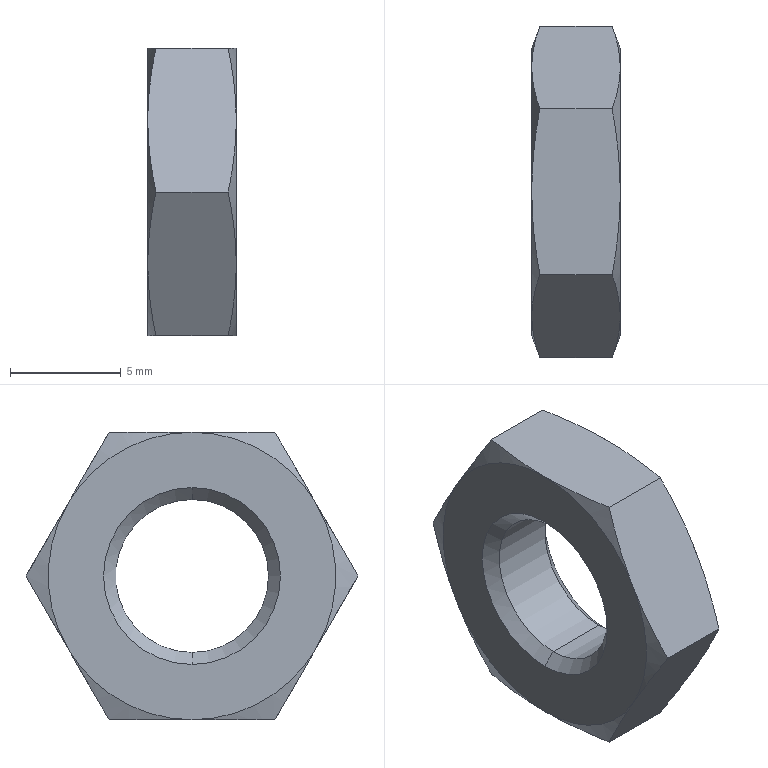Part | 1 solid | 26 faces | box 4 x 15.011 x 13 mm | volume 425.413 mm3 | cone 16 | plane 8 | cylinder 2 | commonest cylinder face diameters 6.917 x2
STEP:
#1=CARTESIAN_POINT('',(0.,0.,0.));
#2=DIRECTION('',(0.,0.,1.));
#3=DIRECTION('',(1.,0.,0.));
#4=AXIS2_PLACEMENT_3D('',#1,#2,#3);
#5=CARTESIAN_POINT('',(-291.373,167.371,-206.624));
#6=VERTEX_POINT('',#5);
#7=CARTESIAN_POINT('',(-291.007,165.494,-203.374));
#8=VERTEX_POINT('',#7);
#9=CARTESIAN_POINT('',(-291.373,167.371,-206.624));
#10=CARTESIAN_POINT('',(-291.373,166.5,-205.116));
#11=CARTESIAN_POINT('',(-291.007,165.494,-203.374));
#12=(BOUNDED_CURVE()B_SPLINE_CURVE(2,(#9,#10,#11),.UNSPECIFIED.,.F.,.U.)B_SPLINE_CURVE_WITH_KNOTS((3,3),(0.,3.786),.UNSPECIFIED.)CURVE()GEOMETRIC_REPRESENTATION_ITEM()RATIONAL_B_SPLINE_CURVE((1.,1.043,1.01))REPRESENTATION_ITEM(''));
#13=EDGE_CURVE('',#6,#8,#12,.T.);
#14=ORIENTED_EDGE('',*,*,#13,.T.);
#15=CARTESIAN_POINT('',(-291.373,167.371,-200.124));
#16=VERTEX_POINT('',#15);
#17=CARTESIAN_POINT('',(-291.007,165.494,-203.374));
#18=CARTESIAN_POINT('',(-291.373,166.5,-201.633));
#19=CARTESIAN_POINT('',(-291.373,167.371,-200.124));
#20=(BOUNDED_CURVE()B_SPLINE_CURVE(2,(#17,#18,#19),.UNSPECIFIED.,.F.,.U.)B_SPLINE_CURVE_WITH_KNOTS((3,3),(0.,3.786),.UNSPECIFIED.)CURVE()GEOMETRIC_REPRESENTATION_ITEM()RATIONAL_B_SPLINE_CURVE((1.01,1.043,1.))REPRESENTATION_ITEM(''));
#21=EDGE_CURVE('',#8,#16,#20,.T.);
#22=ORIENTED_EDGE('',*,*,#21,.T.);
#23=CARTESIAN_POINT('',(-291.373,173.,-203.374));
#24=DIRECTION('',(1.,0.,0.));
#25=DIRECTION('',(0.,-1.,0.));
#26=AXIS2_PLACEMENT_3D('',#23,#24,#25);
#27=CIRCLE('',#26,6.5);
#28=EDGE_CURVE('',#16,#6,#27,.T.);
#29=ORIENTED_EDGE('',*,*,#28,.T.);
#30=EDGE_LOOP('',(#14,#22,#29));
#31=FACE_OUTER_BOUND('',#30,.T.);
#32=CARTESIAN_POINT('',(-291.137,173.,-203.374));
#33=DIRECTION('',(1.,0.,0.));
#34=DIRECTION('',(0.,1.,0.));
#35=AXIS2_PLACEMENT_3D('',#32,#33,#34);
#36=CONICAL_SURFACE('',#35,7.15,1.222);
#37=ADVANCED_FACE('',(#31),#36,.T.);
#38=CARTESIAN_POINT('',(-287.373,167.371,-206.624));
#39=VERTEX_POINT('',#38);
#40=CARTESIAN_POINT('',(-287.739,169.247,-209.874));
#41=VERTEX_POINT('',#40);
#42=CARTESIAN_POINT('',(-287.373,167.371,-206.624));
#43=CARTESIAN_POINT('',(-287.373,168.242,-208.133));
#44=CARTESIAN_POINT('',(-287.739,169.247,-209.874));
#45=(BOUNDED_CURVE()B_SPLINE_CURVE(2,(#42,#43,#44),.UNSPECIFIED.,.F.,.U.)B_SPLINE_CURVE_WITH_KNOTS((3,3),(0.,3.786),.UNSPECIFIED.)CURVE()GEOMETRIC_REPRESENTATION_ITEM()RATIONAL_B_SPLINE_CURVE((1.,1.043,1.01))REPRESENTATION_ITEM(''));
#46=EDGE_CURVE('',#39,#41,#45,.T.);
#47=ORIENTED_EDGE('',*,*,#46,.F.);
#48=CARTESIAN_POINT('',(-287.739,165.494,-203.374));
#49=VERTEX_POINT('',#48);
#50=CARTESIAN_POINT('',(-287.739,165.494,-203.374));
#51=CARTESIAN_POINT('',(-287.373,166.5,-205.116));
#52=CARTESIAN_POINT('',(-287.373,167.371,-206.624));
#53=(BOUNDED_CURVE()B_SPLINE_CURVE(2,(#50,#51,#52),.UNSPECIFIED.,.F.,.U.)B_SPLINE_CURVE_WITH_KNOTS((3,3),(0.,3.786),.UNSPECIFIED.)CURVE()GEOMETRIC_REPRESENTATION_ITEM()RATIONAL_B_SPLINE_CURVE((1.01,1.043,1.))REPRESENTATION_ITEM(''));
#54=EDGE_CURVE('',#49,#39,#53,.T.);
#55=ORIENTED_EDGE('',*,*,#54,.F.);
#56=CARTESIAN_POINT('',(-293.373,165.494,-203.374));
#57=DIRECTION('',(1.,0.,0.));
#58=VECTOR('',#57,1.);
#59=LINE('',#56,#58);
#60=EDGE_CURVE('',#8,#49,#59,.T.);
#61=ORIENTED_EDGE('',*,*,#60,.F.);
#62=ORIENTED_EDGE('',*,*,#13,.F.);
#63=CARTESIAN_POINT('',(-291.007,169.247,-209.874));
#64=VERTEX_POINT('',#63);
#65=CARTESIAN_POINT('',(-291.007,169.247,-209.874));
#66=CARTESIAN_POINT('',(-291.373,168.242,-208.133));
#67=CARTESIAN_POINT('',(-291.373,167.371,-206.624));
#68=(BOUNDED_CURVE()B_SPLINE_CURVE(2,(#65,#66,#67),.UNSPECIFIED.,.F.,.U.)B_SPLINE_CURVE_WITH_KNOTS((3,3),(0.,3.786),.UNSPECIFIED.)CURVE()GEOMETRIC_REPRESENTATION_ITEM()RATIONAL_B_SPLINE_CURVE((1.01,1.043,1.))REPRESENTATION_ITEM(''));
#69=EDGE_CURVE('',#64,#6,#68,.T.);
#70=ORIENTED_EDGE('',*,*,#69,.F.);
#71=CARTESIAN_POINT('',(-293.373,169.247,-209.874));
#72=DIRECTION('',(1.,0.,0.));
#73=VECTOR('',#72,1.);
#74=LINE('',#71,#73);
#75=EDGE_CURVE('',#64,#41,#74,.T.);
#76=ORIENTED_EDGE('',*,*,#75,.T.);
#77=EDGE_LOOP('',(#47,#55,#61,#62,#70,#76));
#78=FACE_OUTER_BOUND('',#77,.T.);
#79=CARTESIAN_POINT('',(-293.373,165.494,-203.374));
#80=DIRECTION('',(0.,0.866,0.5));
#81=DIRECTION('',(0.,-0.5,0.866));
#82=AXIS2_PLACEMENT_3D('',#79,#80,#81);
#83=PLANE('',#82);
#84=ADVANCED_FACE('',(#78),#83,.F.);
#85=CARTESIAN_POINT('',(-287.373,173.,-209.874));
#86=VERTEX_POINT('',#85);
#87=CARTESIAN_POINT('',(-287.739,176.753,-209.874));
#88=VERTEX_POINT('',#87);
#89=CARTESIAN_POINT('',(-287.373,173.,-209.874));
#90=CARTESIAN_POINT('',(-287.373,174.742,-209.874));
#91=CARTESIAN_POINT('',(-287.739,176.753,-209.874));
#92=(BOUNDED_CURVE()B_SPLINE_CURVE(2,(#89,#90,#91),.UNSPECIFIED.,.F.,.U.)B_SPLINE_CURVE_WITH_KNOTS((3,3),(0.,3.786),.UNSPECIFIED.)CURVE()GEOMETRIC_REPRESENTATION_ITEM()RATIONAL_B_SPLINE_CURVE((1.,1.043,1.01))REPRESENTATION_ITEM(''));
#93=EDGE_CURVE('',#86,#88,#92,.T.);
#94=ORIENTED_EDGE('',*,*,#93,.F.);
#95=CARTESIAN_POINT('',(-287.739,169.247,-209.874));
#96=CARTESIAN_POINT('',(-287.373,171.258,-209.874));
#97=CARTESIAN_POINT('',(-287.373,173.,-209.874));
#98=(BOUNDED_CURVE()B_SPLINE_CURVE(2,(#95,#96,#97),.UNSPECIFIED.,.F.,.U.)B_SPLINE_CURVE_WITH_KNOTS((3,3),(0.,3.786),.UNSPECIFIED.)CURVE()GEOMETRIC_REPRESENTATION_ITEM()RATIONAL_B_SPLINE_CURVE((1.01,1.043,1.))REPRESENTATION_ITEM(''));
#99=EDGE_CURVE('',#41,#86,#98,.T.);
#100=ORIENTED_EDGE('',*,*,#99,.F.);
#101=ORIENTED_EDGE('',*,*,#75,.F.);
#102=CARTESIAN_POINT('',(-291.373,173.,-209.874));
#103=VERTEX_POINT('',#102);
#104=CARTESIAN_POINT('',(-291.373,173.,-209.874));
#105=CARTESIAN_POINT('',(-291.373,171.258,-209.874));
#106=CARTESIAN_POINT('',(-291.007,169.247,-209.874));
#107=(BOUNDED_CURVE()B_SPLINE_CURVE(2,(#104,#105,#106),.UNSPECIFIED.,.F.,.U.)B_SPLINE_CURVE_WITH_KNOTS((3,3),(0.,3.786),.UNSPECIFIED.)CURVE()GEOMETRIC_REPRESENTATION_ITEM()RATIONAL_B_SPLINE_CURVE((1.,1.043,1.01))REPRESENTATION_ITEM(''));
#108=EDGE_CURVE('',#103,#64,#107,.T.);
#109=ORIENTED_EDGE('',*,*,#108,.F.);
#110=CARTESIAN_POINT('',(-291.007,176.753,-209.874));
#111=VERTEX_POINT('',#110);
#112=CARTESIAN_POINT('',(-291.007,176.753,-209.874));
#113=CARTESIAN_POINT('',(-291.373,174.742,-209.874));
#114=CARTESIAN_POINT('',(-291.373,173.,-209.874));
#115=(BOUNDED_CURVE()B_SPLINE_CURVE(2,(#112,#113,#114),.UNSPECIFIED.,.F.,.U.)B_SPLINE_CURVE_WITH_KNOTS((3,3),(0.,3.786),.UNSPECIFIED.)CURVE()GEOMETRIC_REPRESENTATION_ITEM()RATIONAL_B_SPLINE_CURVE((1.01,1.043,1.))REPRESENTATION_ITEM(''));
#116=EDGE_CURVE('',#111,#103,#115,.T.);
#117=ORIENTED_EDGE('',*,*,#116,.F.);
#118=CARTESIAN_POINT('',(-293.373,176.753,-209.874));
#119=DIRECTION('',(1.,0.,0.));
#120=VECTOR('',#119,1.);
#121=LINE('',#118,#120);
#122=EDGE_CURVE('',#111,#88,#121,.T.);
#123=ORIENTED_EDGE('',*,*,#122,.T.);
#124=EDGE_LOOP('',(#94,#100,#101,#109,#117,#123));
#125=FACE_OUTER_BOUND('',#124,.T.);
#126=CARTESIAN_POINT('',(-293.373,169.247,-209.874));
#127=DIRECTION('',(0.,0.,1.));
#128=DIRECTION('',(0.,-1.,0.));
#129=AXIS2_PLACEMENT_3D('',#126,#127,#128);
#130=PLANE('',#129);
#131=ADVANCED_FACE('',(#125),#130,.F.);
#132=CARTESIAN_POINT('',(-287.373,178.629,-206.624));
#133=VERTEX_POINT('',#132);
#134=CARTESIAN_POINT('',(-287.739,180.506,-203.374));
#135=VERTEX_POINT('',#134);
#136=CARTESIAN_POINT('',(-287.373,178.629,-206.624));
#137=CARTESIAN_POINT('',(-287.373,179.5,-205.116));
#138=CARTESIAN_POINT('',(-287.739,180.506,-203.374));
#139=(BOUNDED_CURVE()B_SPLINE_CURVE(2,(#136,#137,#138),.UNSPECIFIED.,.F.,.U.)B_SPLINE_CURVE_WITH_KNOTS((3,3),(0.,3.786),.UNSPECIFIED.)CURVE()GEOMETRIC_REPRESENTATION_ITEM()RATIONAL_B_SPLINE_CURVE((1.,1.043,1.01))REPRESENTATION_ITEM(''));
#140=EDGE_CURVE('',#133,#135,#139,.T.);
#141=ORIENTED_EDGE('',*,*,#140,.F.);
#142=CARTESIAN_POINT('',(-287.739,176.753,-209.874));
#143=CARTESIAN_POINT('',(-287.373,177.758,-208.133));
#144=CARTESIAN_POINT('',(-287.373,178.629,-206.624));
#145=(BOUNDED_CURVE()B_SPLINE_CURVE(2,(#142,#143,#144),.UNSPECIFIED.,.F.,.U.)B_SPLINE_CURVE_WITH_KNOTS((3,3),(0.,3.786),.UNSPECIFIED.)CURVE()GEOMETRIC_REPRESENTATION_ITEM()RATIONAL_B_SPLINE_CURVE((1.01,1.043,1.))REPRESENTATION_ITEM(''));
#146=EDGE_CURVE('',#88,#133,#145,.T.);
#147=ORIENTED_EDGE('',*,*,#146,.F.);
#148=ORIENTED_EDGE('',*,*,#122,.F.);
#149=CARTESIAN_POINT('',(-291.373,178.629,-206.624));
#150=VERTEX_POINT('',#149);
#151=CARTESIAN_POINT('',(-291.373,178.629,-206.624));
#152=CARTESIAN_POINT('',(-291.373,177.758,-208.133));
#153=CARTESIAN_POINT('',(-291.007,176.753,-209.874));
#154=(BOUNDED_CURVE()B_SPLINE_CURVE(2,(#151,#152,#153),.UNSPECIFIED.,.F.,.U.)B_SPLINE_CURVE_WITH_KNOTS((3,3),(0.,3.786),.UNSPECIFIED.)CURVE()GEOMETRIC_REPRESENTATION_ITEM()RATIONAL_B_SPLINE_CURVE((1.,1.043,1.01))REPRESENTATION_ITEM(''));
#155=EDGE_CURVE('',#150,#111,#154,.T.);
#156=ORIENTED_EDGE('',*,*,#155,.F.);
#157=CARTESIAN_POINT('',(-291.007,180.506,-203.374));
#158=VERTEX_POINT('',#157);
#159=CARTESIAN_POINT('',(-291.007,180.506,-203.374));
#160=CARTESIAN_POINT('',(-291.373,179.5,-205.116));
#161=CARTESIAN_POINT('',(-291.373,178.629,-206.624));
#162=(BOUNDED_CURVE()B_SPLINE_CURVE(2,(#159,#160,#161),.UNSPECIFIED.,.F.,.U.)B_SPLINE_CURVE_WITH_KNOTS((3,3),(0.,3.786),.UNSPECIFIED.)CURVE()GEOMETRIC_REPRESENTATION_ITEM()RATIONAL_B_SPLINE_CURVE((1.01,1.043,1.))REPRESENTATION_ITEM(''));
#163=EDGE_CURVE('',#158,#150,#162,.T.);
#164=ORIENTED_EDGE('',*,*,#163,.F.);
#165=CARTESIAN_POINT('',(-293.373,180.506,-203.374));
#166=DIRECTION('',(1.,0.,0.));
#167=VECTOR('',#166,1.);
#168=LINE('',#165,#167);
#169=EDGE_CURVE('',#158,#135,#168,.T.);
#170=ORIENTED_EDGE('',*,*,#169,.T.);
#171=EDGE_LOOP('',(#141,#147,#148,#156,#164,#170));
#172=FACE_OUTER_BOUND('',#171,.T.);
#173=CARTESIAN_POINT('',(-293.373,176.753,-209.874));
#174=DIRECTION('',(0.,-0.866,0.5));
#175=DIRECTION('',(0.,-0.5,-0.866));
#176=AXIS2_PLACEMENT_3D('',#173,#174,#175);
#177=PLANE('',#176);
#178=ADVANCED_FACE('',(#172),#177,.F.);
#179=CARTESIAN_POINT('',(-287.373,178.629,-200.124));
#180=VERTEX_POINT('',#179);
#181=CARTESIAN_POINT('',(-287.739,180.506,-203.374));
#182=CARTESIAN_POINT('',(-287.373,179.5,-201.633));
#183=CARTESIAN_POINT('',(-287.373,178.629,-200.124));
#184=(BOUNDED_CURVE()B_SPLINE_CURVE(2,(#181,#182,#183),.UNSPECIFIED.,.F.,.U.)B_SPLINE_CURVE_WITH_KNOTS((3,3),(0.,3.786),.UNSPECIFIED.)CURVE()GEOMETRIC_REPRESENTATION_ITEM()RATIONAL_B_SPLINE_CURVE((1.01,1.043,1.))REPRESENTATION_ITEM(''));
#185=EDGE_CURVE('',#135,#180,#184,.T.);
#186=ORIENTED_EDGE('',*,*,#185,.F.);
#187=ORIENTED_EDGE('',*,*,#169,.F.);
#188=CARTESIAN_POINT('',(-291.373,178.629,-200.124));
#189=VERTEX_POINT('',#188);
#190=CARTESIAN_POINT('',(-291.373,178.629,-200.124));
#191=CARTESIAN_POINT('',(-291.373,179.5,-201.633));
#192=CARTESIAN_POINT('',(-291.007,180.506,-203.374));
#193=(BOUNDED_CURVE()B_SPLINE_CURVE(2,(#190,#191,#192),.UNSPECIFIED.,.F.,.U.)B_SPLINE_CURVE_WITH_KNOTS((3,3),(0.,3.786),.UNSPECIFIED.)CURVE()GEOMETRIC_REPRESENTATION_ITEM()RATIONAL_B_SPLINE_CURVE((1.,1.043,1.01))REPRESENTATION_ITEM(''));
#194=EDGE_CURVE('',#189,#158,#193,.T.);
#195=ORIENTED_EDGE('',*,*,#194,.F.);
#196=CARTESIAN_POINT('',(-291.007,176.753,-196.874));
#197=VERTEX_POINT('',#196);
#198=CARTESIAN_POINT('',(-291.007,176.753,-196.874));
#199=CARTESIAN_POINT('',(-291.373,177.758,-198.616));
#200=CARTESIAN_POINT('',(-291.373,178.629,-200.124));
#201=(BOUNDED_CURVE()B_SPLINE_CURVE(2,(#198,#199,#200),.UNSPECIFIED.,.F.,.U.)B_SPLINE_CURVE_WITH_KNOTS((3,3),(0.,3.786),.UNSPECIFIED.)CURVE()GEOMETRIC_REPRESENTATION_ITEM()RATIONAL_B_SPLINE_CURVE((1.01,1.043,1.))REPRESENTATION_ITEM(''));
#202=EDGE_CURVE('',#197,#189,#201,.T.);
#203=ORIENTED_EDGE('',*,*,#202,.F.);
#204=CARTESIAN_POINT('',(-287.739,176.753,-196.874));
#205=VERTEX_POINT('',#204);
#206=CARTESIAN_POINT('',(-293.373,176.753,-196.874));
#207=DIRECTION('',(1.,0.,0.));
#208=VECTOR('',#207,1.);
#209=LINE('',#206,#208);
#210=EDGE_CURVE('',#197,#205,#209,.T.);
#211=ORIENTED_EDGE('',*,*,#210,.T.);
#212=CARTESIAN_POINT('',(-287.373,178.629,-200.124));
#213=CARTESIAN_POINT('',(-287.373,177.758,-198.616));
#214=CARTESIAN_POINT('',(-287.739,176.753,-196.874));
#215=(BOUNDED_CURVE()B_SPLINE_CURVE(2,(#212,#213,#214),.UNSPECIFIED.,.F.,.U.)B_SPLINE_CURVE_WITH_KNOTS((3,3),(0.,3.786),.UNSPECIFIED.)CURVE()GEOMETRIC_REPRESENTATION_ITEM()RATIONAL_B_SPLINE_CURVE((1.,1.043,1.01))REPRESENTATION_ITEM(''));
#216=EDGE_CURVE('',#180,#205,#215,.T.);
#217=ORIENTED_EDGE('',*,*,#216,.F.);
#218=EDGE_LOOP('',(#186,#187,#195,#203,#211,#217));
#219=FACE_OUTER_BOUND('',#218,.T.);
#220=CARTESIAN_POINT('',(-293.373,180.506,-203.374));
#221=DIRECTION('',(0.,-0.866,-0.5));
#222=DIRECTION('',(0.,0.5,-0.866));
#223=AXIS2_PLACEMENT_3D('',#220,#221,#222);
#224=PLANE('',#223);
#225=ADVANCED_FACE('',(#219),#224,.F.);
#226=ORIENTED_EDGE('',*,*,#216,.T.);
#227=CARTESIAN_POINT('',(-287.373,173.,-196.874));
#228=VERTEX_POINT('',#227);
#229=CARTESIAN_POINT('',(-287.739,176.753,-196.874));
#230=CARTESIAN_POINT('',(-287.373,174.742,-196.874));
#231=CARTESIAN_POINT('',(-287.373,173.,-196.874));
#232=(BOUNDED_CURVE()B_SPLINE_CURVE(2,(#229,#230,#231),.UNSPECIFIED.,.F.,.U.)B_SPLINE_CURVE_WITH_KNOTS((3,3),(0.,3.786),.UNSPECIFIED.)CURVE()GEOMETRIC_REPRESENTATION_ITEM()RATIONAL_B_SPLINE_CURVE((1.01,1.043,1.))REPRESENTATION_ITEM(''));
#233=EDGE_CURVE('',#205,#228,#232,.T.);
#234=ORIENTED_EDGE('',*,*,#233,.T.);
#235=CARTESIAN_POINT('',(-287.373,173.,-203.374));
#236=DIRECTION('',(1.,0.,0.));
#237=DIRECTION('',(0.,-1.,0.));
#238=AXIS2_PLACEMENT_3D('',#235,#236,#237);
#239=CIRCLE('',#238,6.5);
#240=EDGE_CURVE('',#180,#228,#239,.T.);
#241=ORIENTED_EDGE('',*,*,#240,.F.);
#242=EDGE_LOOP('',(#226,#234,#241));
#243=FACE_OUTER_BOUND('',#242,.T.);
#244=CARTESIAN_POINT('',(-287.61,173.,-203.374));
#245=DIRECTION('',(-1.,0.,0.));
#246=DIRECTION('',(0.,-0.5,-0.866));
#247=AXIS2_PLACEMENT_3D('',#244,#245,#246);
#248=CONICAL_SURFACE('',#247,7.15,1.222);
#249=ADVANCED_FACE('',(#243),#248,.T.);
#250=CARTESIAN_POINT('',(-287.373,169.,-203.374));
#251=VERTEX_POINT('',#250);
#252=CARTESIAN_POINT('',(-287.373,173.,-199.374));
#253=VERTEX_POINT('',#252);
#254=CARTESIAN_POINT('',(-287.373,173.,-203.374));
#255=DIRECTION('',(-1.,0.,0.));
#256=DIRECTION('',(0.,-1.,0.));
#257=AXIS2_PLACEMENT_3D('',#254,#255,#256);
#258=CIRCLE('',#257,4.);
#259=EDGE_CURVE('',#251,#253,#258,.T.);
#260=ORIENTED_EDGE('',*,*,#259,.T.);
#261=CARTESIAN_POINT('',(-287.373,173.,-207.374));
#262=VERTEX_POINT('',#261);
#263=CARTESIAN_POINT('',(-287.373,173.,-203.374));
#264=DIRECTION('',(-1.,0.,0.));
#265=DIRECTION('',(0.,-1.,0.));
#266=AXIS2_PLACEMENT_3D('',#263,#264,#265);
#267=CIRCLE('',#266,4.);
#268=EDGE_CURVE('',#253,#262,#267,.T.);
#269=ORIENTED_EDGE('',*,*,#268,.T.);
#270=CARTESIAN_POINT('',(-287.373,173.,-203.374));
#271=DIRECTION('',(-1.,0.,0.));
#272=DIRECTION('',(0.,-1.,0.));
#273=AXIS2_PLACEMENT_3D('',#270,#271,#272);
#274=CIRCLE('',#273,4.);
#275=EDGE_CURVE('',#262,#251,#274,.T.);
#276=ORIENTED_EDGE('',*,*,#275,.T.);
#277=EDGE_LOOP('',(#260,#269,#276));
#278=FACE_BOUND('',#277,.T.);
#279=CARTESIAN_POINT('',(-287.373,167.371,-200.124));
#280=VERTEX_POINT('',#279);
#281=CARTESIAN_POINT('',(-287.373,173.,-203.374));
#282=DIRECTION('',(1.,0.,0.));
#283=DIRECTION('',(0.,-1.,0.));
#284=AXIS2_PLACEMENT_3D('',#281,#282,#283);
#285=CIRCLE('',#284,6.5);
#286=EDGE_CURVE('',#228,#280,#285,.T.);
#287=ORIENTED_EDGE('',*,*,#286,.T.);
#288=CARTESIAN_POINT('',(-287.373,173.,-203.374));
#289=DIRECTION('',(1.,0.,0.));
#290=DIRECTION('',(0.,-1.,0.));
#291=AXIS2_PLACEMENT_3D('',#288,#289,#290);
#292=CIRCLE('',#291,6.5);
#293=EDGE_CURVE('',#280,#39,#292,.T.);
#294=ORIENTED_EDGE('',*,*,#293,.T.);
#295=CARTESIAN_POINT('',(-287.373,173.,-203.374));
#296=DIRECTION('',(1.,0.,0.));
#297=DIRECTION('',(0.,-1.,0.));
#298=AXIS2_PLACEMENT_3D('',#295,#296,#297);
#299=CIRCLE('',#298,6.5);
#300=EDGE_CURVE('',#39,#86,#299,.T.);
#301=ORIENTED_EDGE('',*,*,#300,.T.);
#302=CARTESIAN_POINT('',(-287.373,173.,-203.374));
#303=DIRECTION('',(1.,0.,0.));
#304=DIRECTION('',(0.,-1.,0.));
#305=AXIS2_PLACEMENT_3D('',#302,#303,#304);
#306=CIRCLE('',#305,6.5);
#307=EDGE_CURVE('',#86,#133,#306,.T.);
#308=ORIENTED_EDGE('',*,*,#307,.T.);
#309=CARTESIAN_POINT('',(-287.373,173.,-203.374));
#310=DIRECTION('',(1.,0.,0.));
#311=DIRECTION('',(0.,-1.,0.));
#312=AXIS2_PLACEMENT_3D('',#309,#310,#311);
#313=CIRCLE('',#312,6.5);
#314=EDGE_CURVE('',#133,#180,#313,.T.);
#315=ORIENTED_EDGE('',*,*,#314,.T.);
#316=ORIENTED_EDGE('',*,*,#240,.T.);
#317=EDGE_LOOP('',(#287,#294,#301,#308,#315,#316));
#318=FACE_OUTER_BOUND('',#317,.T.);
#319=CARTESIAN_POINT('',(-287.373,169.75,-203.374));
#320=DIRECTION('',(1.,0.,0.));
#321=DIRECTION('',(0.,-1.,0.));
#322=AXIS2_PLACEMENT_3D('',#319,#320,#321);
#323=PLANE('',#322);
#324=ADVANCED_FACE('',(#278,#318),#323,.T.);
#325=CARTESIAN_POINT('',(-287.739,169.247,-196.874));
#326=VERTEX_POINT('',#325);
#327=CARTESIAN_POINT('',(-287.373,173.,-196.874));
#328=CARTESIAN_POINT('',(-287.373,171.258,-196.874));
#329=CARTESIAN_POINT('',(-287.739,169.247,-196.874));
#330=(BOUNDED_CURVE()B_SPLINE_CURVE(2,(#327,#328,#329),.UNSPECIFIED.,.F.,.U.)B_SPLINE_CURVE_WITH_KNOTS((3,3),(0.,3.786),.UNSPECIFIED.)CURVE()GEOMETRIC_REPRESENTATION_ITEM()RATIONAL_B_SPLINE_CURVE((1.,1.043,1.01))REPRESENTATION_ITEM(''));
#331=EDGE_CURVE('',#228,#326,#330,.T.);
#332=ORIENTED_EDGE('',*,*,#331,.T.);
#333=CARTESIAN_POINT('',(-287.739,169.247,-196.874));
#334=CARTESIAN_POINT('',(-287.373,168.242,-198.616));
#335=CARTESIAN_POINT('',(-287.373,167.371,-200.124));
#336=(BOUNDED_CURVE()B_SPLINE_CURVE(2,(#333,#334,#335),.UNSPECIFIED.,.F.,.U.)B_SPLINE_CURVE_WITH_KNOTS((3,3),(0.,3.786),.UNSPECIFIED.)CURVE()GEOMETRIC_REPRESENTATION_ITEM()RATIONAL_B_SPLINE_CURVE((1.01,1.043,1.))REPRESENTATION_ITEM(''));
#337=EDGE_CURVE('',#326,#280,#336,.T.);
#338=ORIENTED_EDGE('',*,*,#337,.T.);
#339=ORIENTED_EDGE('',*,*,#286,.F.);
#340=EDGE_LOOP('',(#332,#338,#339));
#341=FACE_OUTER_BOUND('',#340,.T.);
#342=CARTESIAN_POINT('',(-287.61,173.,-203.374));
#343=DIRECTION('',(-1.,0.,0.));
#344=DIRECTION('',(0.,0.5,-0.866));
#345=AXIS2_PLACEMENT_3D('',#342,#343,#344);
#346=CONICAL_SURFACE('',#345,7.15,1.222);
#347=ADVANCED_FACE('',(#341),#346,.T.);
#348=ORIENTED_EDGE('',*,*,#337,.F.);
#349=CARTESIAN_POINT('',(-291.007,169.247,-196.874));
#350=VERTEX_POINT('',#349);
#351=CARTESIAN_POINT('',(-293.373,169.247,-196.874));
#352=DIRECTION('',(1.,0.,0.));
#353=VECTOR('',#352,1.);
#354=LINE('',#351,#353);
#355=EDGE_CURVE('',#350,#326,#354,.T.);
#356=ORIENTED_EDGE('',*,*,#355,.F.);
#357=CARTESIAN_POINT('',(-291.373,167.371,-200.124));
#358=CARTESIAN_POINT('',(-291.373,168.242,-198.616));
#359=CARTESIAN_POINT('',(-291.007,169.247,-196.874));
#360=(BOUNDED_CURVE()B_SPLINE_CURVE(2,(#357,#358,#359),.UNSPECIFIED.,.F.,.U.)B_SPLINE_CURVE_WITH_KNOTS((3,3),(0.,3.786),.UNSPECIFIED.)CURVE()GEOMETRIC_REPRESENTATION_ITEM()RATIONAL_B_SPLINE_CURVE((1.,1.043,1.01))REPRESENTATION_ITEM(''));
#361=EDGE_CURVE('',#16,#350,#360,.T.);
#362=ORIENTED_EDGE('',*,*,#361,.F.);
#363=ORIENTED_EDGE('',*,*,#21,.F.);
#364=ORIENTED_EDGE('',*,*,#60,.T.);
#365=CARTESIAN_POINT('',(-287.373,167.371,-200.124));
#366=CARTESIAN_POINT('',(-287.373,166.5,-201.633));
#367=CARTESIAN_POINT('',(-287.739,165.494,-203.374));
#368=(BOUNDED_CURVE()B_SPLINE_CURVE(2,(#365,#366,#367),.UNSPECIFIED.,.F.,.U.)B_SPLINE_CURVE_WITH_KNOTS((3,3),(0.,3.786),.UNSPECIFIED.)CURVE()GEOMETRIC_REPRESENTATION_ITEM()RATIONAL_B_SPLINE_CURVE((1.,1.043,1.01))REPRESENTATION_ITEM(''));
#369=EDGE_CURVE('',#280,#49,#368,.T.);
#370=ORIENTED_EDGE('',*,*,#369,.F.);
#371=EDGE_LOOP('',(#348,#356,#362,#363,#364,#370));
#372=FACE_OUTER_BOUND('',#371,.T.);
#373=CARTESIAN_POINT('',(-293.373,169.247,-196.874));
#374=DIRECTION('',(0.,0.866,-0.5));
#375=DIRECTION('',(0.,0.5,0.866));
#376=AXIS2_PLACEMENT_3D('',#373,#374,#375);
#377=PLANE('',#376);
#378=ADVANCED_FACE('',(#372),#377,.F.);
#379=ORIENTED_EDGE('',*,*,#293,.F.);
#380=ORIENTED_EDGE('',*,*,#369,.T.);
#381=ORIENTED_EDGE('',*,*,#54,.T.);
#382=EDGE_LOOP('',(#379,#380,#381));
#383=FACE_OUTER_BOUND('',#382,.T.);
#384=CARTESIAN_POINT('',(-287.61,173.,-203.374));
#385=DIRECTION('',(-1.,0.,0.));
#386=DIRECTION('',(0.,1.,0.));
#387=AXIS2_PLACEMENT_3D('',#384,#385,#386);
#388=CONICAL_SURFACE('',#387,7.15,1.222);
#389=ADVANCED_FACE('',(#383),#388,.T.);
#390=CARTESIAN_POINT('',(-291.373,169.,-203.374));
#391=VERTEX_POINT('',#390);
#392=CARTESIAN_POINT('',(-291.373,173.,-207.374));
#393=VERTEX_POINT('',#392);
#394=CARTESIAN_POINT('',(-291.373,173.,-203.374));
#395=DIRECTION('',(1.,0.,0.));
#396=DIRECTION('',(0.,-1.,0.));
#397=AXIS2_PLACEMENT_3D('',#394,#395,#396);
#398=CIRCLE('',#397,4.);
#399=EDGE_CURVE('',#391,#393,#398,.T.);
#400=ORIENTED_EDGE('',*,*,#399,.T.);
#401=CARTESIAN_POINT('',(-291.373,173.,-199.374));
#402=VERTEX_POINT('',#401);
#403=CARTESIAN_POINT('',(-291.373,173.,-203.374));
#404=DIRECTION('',(1.,0.,0.));
#405=DIRECTION('',(0.,-1.,0.));
#406=AXIS2_PLACEMENT_3D('',#403,#404,#405);
#407=CIRCLE('',#406,4.);
#408=EDGE_CURVE('',#393,#402,#407,.T.);
#409=ORIENTED_EDGE('',*,*,#408,.T.);
#410=CARTESIAN_POINT('',(-291.373,173.,-203.374));
#411=DIRECTION('',(1.,0.,0.));
#412=DIRECTION('',(0.,-1.,0.));
#413=AXIS2_PLACEMENT_3D('',#410,#411,#412);
#414=CIRCLE('',#413,4.);
#415=EDGE_CURVE('',#402,#391,#414,.T.);
#416=ORIENTED_EDGE('',*,*,#415,.T.);
#417=EDGE_LOOP('',(#400,#409,#416));
#418=FACE_BOUND('',#417,.T.);
#419=ORIENTED_EDGE('',*,*,#28,.F.);
#420=CARTESIAN_POINT('',(-291.373,173.,-196.874));
#421=VERTEX_POINT('',#420);
#422=CARTESIAN_POINT('',(-291.373,173.,-203.374));
#423=DIRECTION('',(1.,0.,0.));
#424=DIRECTION('',(0.,-1.,0.));
#425=AXIS2_PLACEMENT_3D('',#422,#423,#424);
#426=CIRCLE('',#425,6.5);
#427=EDGE_CURVE('',#421,#16,#426,.T.);
#428=ORIENTED_EDGE('',*,*,#427,.F.);
#429=CARTESIAN_POINT('',(-291.373,173.,-203.374));
#430=DIRECTION('',(1.,0.,0.));
#431=DIRECTION('',(0.,-1.,0.));
#432=AXIS2_PLACEMENT_3D('',#429,#430,#431);
#433=CIRCLE('',#432,6.5);
#434=EDGE_CURVE('',#189,#421,#433,.T.);
#435=ORIENTED_EDGE('',*,*,#434,.F.);
#436=CARTESIAN_POINT('',(-291.373,173.,-203.374));
#437=DIRECTION('',(1.,0.,0.));
#438=DIRECTION('',(0.,-1.,0.));
#439=AXIS2_PLACEMENT_3D('',#436,#437,#438);
#440=CIRCLE('',#439,6.5);
#441=EDGE_CURVE('',#150,#189,#440,.T.);
#442=ORIENTED_EDGE('',*,*,#441,.F.);
#443=CARTESIAN_POINT('',(-291.373,173.,-203.374));
#444=DIRECTION('',(1.,0.,0.));
#445=DIRECTION('',(0.,-1.,0.));
#446=AXIS2_PLACEMENT_3D('',#443,#444,#445);
#447=CIRCLE('',#446,6.5);
#448=EDGE_CURVE('',#103,#150,#447,.T.);
#449=ORIENTED_EDGE('',*,*,#448,.F.);
#450=CARTESIAN_POINT('',(-291.373,173.,-203.374));
#451=DIRECTION('',(1.,0.,0.));
#452=DIRECTION('',(0.,-1.,0.));
#453=AXIS2_PLACEMENT_3D('',#450,#451,#452);
#454=CIRCLE('',#453,6.5);
#455=EDGE_CURVE('',#6,#103,#454,.T.);
#456=ORIENTED_EDGE('',*,*,#455,.F.);
#457=EDGE_LOOP('',(#419,#428,#435,#442,#449,#456));
#458=FACE_OUTER_BOUND('',#457,.T.);
#459=CARTESIAN_POINT('',(-291.373,169.75,-203.374));
#460=DIRECTION('',(-1.,0.,0.));
#461=DIRECTION('',(0.,1.,0.));
#462=AXIS2_PLACEMENT_3D('',#459,#460,#461);
#463=PLANE('',#462);
#464=ADVANCED_FACE('',(#418,#458),#463,.T.);
#465=ORIENTED_EDGE('',*,*,#108,.T.);
#466=ORIENTED_EDGE('',*,*,#69,.T.);
#467=ORIENTED_EDGE('',*,*,#455,.T.);
#468=EDGE_LOOP('',(#465,#466,#467));
#469=FACE_OUTER_BOUND('',#468,.T.);
#470=CARTESIAN_POINT('',(-291.137,173.,-203.374));
#471=DIRECTION('',(1.,0.,0.));
#472=DIRECTION('',(0.,0.5,0.866));
#473=AXIS2_PLACEMENT_3D('',#470,#471,#472);
#474=CONICAL_SURFACE('',#473,7.15,1.222);
#475=ADVANCED_FACE('',(#469),#474,.T.);
#476=ORIENTED_EDGE('',*,*,#116,.T.);
#477=ORIENTED_EDGE('',*,*,#448,.T.);
#478=ORIENTED_EDGE('',*,*,#155,.T.);
#479=EDGE_LOOP('',(#476,#477,#478));
#480=FACE_OUTER_BOUND('',#479,.T.);
#481=CARTESIAN_POINT('',(-291.137,173.,-203.374));
#482=DIRECTION('',(1.,0.,0.));
#483=DIRECTION('',(0.,-0.5,0.866));
#484=AXIS2_PLACEMENT_3D('',#481,#482,#483);
#485=CONICAL_SURFACE('',#484,7.15,1.222);
#486=ADVANCED_FACE('',(#480),#485,.T.);
#487=ORIENTED_EDGE('',*,*,#441,.T.);
#488=ORIENTED_EDGE('',*,*,#194,.T.);
#489=ORIENTED_EDGE('',*,*,#163,.T.);
#490=EDGE_LOOP('',(#487,#488,#489));
#491=FACE_OUTER_BOUND('',#490,.T.);
#492=CARTESIAN_POINT('',(-291.137,173.,-203.374));
#493=DIRECTION('',(1.,0.,0.));
#494=DIRECTION('',(0.,-1.,0.));
#495=AXIS2_PLACEMENT_3D('',#492,#493,#494);
#496=CONICAL_SURFACE('',#495,7.15,1.222);
#497=ADVANCED_FACE('',(#491),#496,.T.);
#498=ORIENTED_EDGE('',*,*,#202,.T.);
#499=ORIENTED_EDGE('',*,*,#434,.T.);
#500=CARTESIAN_POINT('',(-291.373,173.,-196.874));
#501=CARTESIAN_POINT('',(-291.373,174.742,-196.874));
#502=CARTESIAN_POINT('',(-291.007,176.753,-196.874));
#503=(BOUNDED_CURVE()B_SPLINE_CURVE(2,(#500,#501,#502),.UNSPECIFIED.,.F.,.U.)B_SPLINE_CURVE_WITH_KNOTS((3,3),(0.,3.786),.UNSPECIFIED.)CURVE()GEOMETRIC_REPRESENTATION_ITEM()RATIONAL_B_SPLINE_CURVE((1.,1.043,1.01))REPRESENTATION_ITEM(''));
#504=EDGE_CURVE('',#421,#197,#503,.T.);
#505=ORIENTED_EDGE('',*,*,#504,.T.);
#506=EDGE_LOOP('',(#498,#499,#505));
#507=FACE_OUTER_BOUND('',#506,.T.);
#508=CARTESIAN_POINT('',(-291.137,173.,-203.374));
#509=DIRECTION('',(1.,0.,0.));
#510=DIRECTION('',(0.,-0.5,-0.866));
#511=AXIS2_PLACEMENT_3D('',#508,#509,#510);
#512=CONICAL_SURFACE('',#511,7.15,1.222);
#513=ADVANCED_FACE('',(#507),#512,.T.);
#514=ORIENTED_EDGE('',*,*,#233,.F.);
#515=ORIENTED_EDGE('',*,*,#210,.F.);
#516=ORIENTED_EDGE('',*,*,#504,.F.);
#517=CARTESIAN_POINT('',(-291.007,169.247,-196.874));
#518=CARTESIAN_POINT('',(-291.373,171.258,-196.874));
#519=CARTESIAN_POINT('',(-291.373,173.,-196.874));
#520=(BOUNDED_CURVE()B_SPLINE_CURVE(2,(#517,#518,#519),.UNSPECIFIED.,.F.,.U.)B_SPLINE_CURVE_WITH_KNOTS((3,3),(0.,3.786),.UNSPECIFIED.)CURVE()GEOMETRIC_REPRESENTATION_ITEM()RATIONAL_B_SPLINE_CURVE((1.01,1.043,1.))REPRESENTATION_ITEM(''));
#521=EDGE_CURVE('',#350,#421,#520,.T.);
#522=ORIENTED_EDGE('',*,*,#521,.F.);
#523=ORIENTED_EDGE('',*,*,#355,.T.);
#524=ORIENTED_EDGE('',*,*,#331,.F.);
#525=EDGE_LOOP('',(#514,#515,#516,#522,#523,#524));
#526=FACE_OUTER_BOUND('',#525,.T.);
#527=CARTESIAN_POINT('',(-293.373,176.753,-196.874));
#528=DIRECTION('',(0.,0.,-1.));
#529=DIRECTION('',(0.,1.,0.));
#530=AXIS2_PLACEMENT_3D('',#527,#528,#529);
#531=PLANE('',#530);
#532=ADVANCED_FACE('',(#526),#531,.F.);
#533=ORIENTED_EDGE('',*,*,#361,.T.);
#534=ORIENTED_EDGE('',*,*,#521,.T.);
#535=ORIENTED_EDGE('',*,*,#427,.T.);
#536=EDGE_LOOP('',(#533,#534,#535));
#537=FACE_OUTER_BOUND('',#536,.T.);
#538=CARTESIAN_POINT('',(-291.137,173.,-203.374));
#539=DIRECTION('',(1.,0.,0.));
#540=DIRECTION('',(0.,0.5,-0.866));
#541=AXIS2_PLACEMENT_3D('',#538,#539,#540);
#542=CONICAL_SURFACE('',#541,7.15,1.222);
#543=ADVANCED_FACE('',(#537),#542,.T.);
#544=CARTESIAN_POINT('',(-287.915,173.,-206.833));
#545=VERTEX_POINT('',#544);
#546=CARTESIAN_POINT('',(-287.915,173.,-206.833));
#547=DIRECTION('',(0.7071,0.,-0.7071));
#548=VECTOR('',#547,1.);
#549=LINE('',#546,#548);
#550=EDGE_CURVE('',#545,#262,#549,.T.);
#551=ORIENTED_EDGE('',*,*,#550,.T.);
#552=ORIENTED_EDGE('',*,*,#268,.F.);
#553=CARTESIAN_POINT('',(-287.915,173.,-199.916));
#554=VERTEX_POINT('',#553);
#555=CARTESIAN_POINT('',(-287.915,173.,-199.916));
#556=DIRECTION('',(0.7071,0.,0.7071));
#557=VECTOR('',#556,1.);
#558=LINE('',#555,#557);
#559=EDGE_CURVE('',#554,#253,#558,.T.);
#560=ORIENTED_EDGE('',*,*,#559,.F.);
#561=CARTESIAN_POINT('',(-287.915,173.,-203.374));
#562=DIRECTION('',(1.,0.,0.));
#563=DIRECTION('',(0.,-1.,0.));
#564=AXIS2_PLACEMENT_3D('',#561,#562,#563);
#565=CIRCLE('',#564,3.458);
#566=EDGE_CURVE('',#545,#554,#565,.T.);
#567=ORIENTED_EDGE('',*,*,#566,.F.);
#568=EDGE_LOOP('',(#551,#552,#560,#567));
#569=FACE_OUTER_BOUND('',#568,.T.);
#570=CARTESIAN_POINT('',(-287.644,173.,-203.374));
#571=DIRECTION('',(1.,0.,0.));
#572=DIRECTION('',(0.,-1.,0.));
#573=AXIS2_PLACEMENT_3D('',#570,#571,#572);
#574=CONICAL_SURFACE('',#573,3.729,0.7854);
#575=ADVANCED_FACE('',(#569),#574,.F.);
#576=CARTESIAN_POINT('',(-290.832,173.,-206.833));
#577=VERTEX_POINT('',#576);
#578=CARTESIAN_POINT('',(-287.915,173.,-206.833));
#579=DIRECTION('',(-1.,-0.000000001,0.));
#580=VECTOR('',#579,1.);
#581=LINE('',#578,#580);
#582=EDGE_CURVE('',#545,#577,#581,.T.);
#583=ORIENTED_EDGE('',*,*,#582,.T.);
#584=CARTESIAN_POINT('',(-290.832,169.541,-203.374));
#585=VERTEX_POINT('',#584);
#586=CARTESIAN_POINT('',(-290.832,173.,-203.374));
#587=DIRECTION('',(1.,0.,0.));
#588=DIRECTION('',(0.,-1.,0.));
#589=AXIS2_PLACEMENT_3D('',#586,#587,#588);
#590=CIRCLE('',#589,3.458);
#591=EDGE_CURVE('',#585,#577,#590,.T.);
#592=ORIENTED_EDGE('',*,*,#591,.F.);
#593=CARTESIAN_POINT('',(-290.832,173.,-199.916));
#594=VERTEX_POINT('',#593);
#595=CARTESIAN_POINT('',(-290.832,173.,-203.374));
#596=DIRECTION('',(1.,0.,0.));
#597=DIRECTION('',(0.,-1.,0.));
#598=AXIS2_PLACEMENT_3D('',#595,#596,#597);
#599=CIRCLE('',#598,3.458);
#600=EDGE_CURVE('',#594,#585,#599,.T.);
#601=ORIENTED_EDGE('',*,*,#600,.F.);
#602=CARTESIAN_POINT('',(-287.915,173.,-199.916));
#603=DIRECTION('',(-1.,0.,0.));
#604=VECTOR('',#603,1.);
#605=LINE('',#602,#604);
#606=EDGE_CURVE('',#554,#594,#605,.T.);
#607=ORIENTED_EDGE('',*,*,#606,.F.);
#608=CARTESIAN_POINT('',(-287.915,169.541,-203.374));
#609=VERTEX_POINT('',#608);
#610=CARTESIAN_POINT('',(-287.915,173.,-203.374));
#611=DIRECTION('',(1.,0.,0.));
#612=DIRECTION('',(0.,-1.,0.));
#613=AXIS2_PLACEMENT_3D('',#610,#611,#612);
#614=CIRCLE('',#613,3.458);
#615=EDGE_CURVE('',#554,#609,#614,.T.);
#616=ORIENTED_EDGE('',*,*,#615,.T.);
#617=CARTESIAN_POINT('',(-287.915,173.,-203.374));
#618=DIRECTION('',(1.,0.,0.));
#619=DIRECTION('',(0.,-1.,0.));
#620=AXIS2_PLACEMENT_3D('',#617,#618,#619);
#621=CIRCLE('',#620,3.458);
#622=EDGE_CURVE('',#609,#545,#621,.T.);
#623=ORIENTED_EDGE('',*,*,#622,.T.);
#624=EDGE_LOOP('',(#583,#592,#601,#607,#616,#623));
#625=FACE_OUTER_BOUND('',#624,.T.);
#626=CARTESIAN_POINT('',(-289.373,173.,-203.374));
#627=DIRECTION('',(-1.,0.,0.));
#628=DIRECTION('',(0.,1.,-0.000000001));
#629=AXIS2_PLACEMENT_3D('',#626,#627,#628);
#630=CYLINDRICAL_SURFACE('',#629,3.458);
#631=ADVANCED_FACE('',(#625),#630,.F.);
#632=CARTESIAN_POINT('',(-290.832,173.,-206.833));
#633=DIRECTION('',(-0.7071,0.000000004,-0.7071));
#634=VECTOR('',#633,1.);
#635=LINE('',#632,#634);
#636=EDGE_CURVE('',#577,#393,#635,.T.);
#637=ORIENTED_EDGE('',*,*,#636,.T.);
#638=ORIENTED_EDGE('',*,*,#399,.F.);
#639=ORIENTED_EDGE('',*,*,#415,.F.);
#640=CARTESIAN_POINT('',(-290.832,173.,-199.916));
#641=DIRECTION('',(-0.7071,0.,0.7071));
#642=VECTOR('',#641,1.);
#643=LINE('',#640,#642);
#644=EDGE_CURVE('',#594,#402,#643,.T.);
#645=ORIENTED_EDGE('',*,*,#644,.F.);
#646=ORIENTED_EDGE('',*,*,#600,.T.);
#647=ORIENTED_EDGE('',*,*,#591,.T.);
#648=EDGE_LOOP('',(#637,#638,#639,#645,#646,#647));
#649=FACE_OUTER_BOUND('',#648,.T.);
#650=CARTESIAN_POINT('',(-291.102,173.,-203.374));
#651=DIRECTION('',(-1.,0.,0.));
#652=DIRECTION('',(0.,1.,0.));
#653=AXIS2_PLACEMENT_3D('',#650,#651,#652);
#654=CONICAL_SURFACE('',#653,3.729,0.7854);
#655=ADVANCED_FACE('',(#649),#654,.F.);
#656=ORIENTED_EDGE('',*,*,#140,.T.);
#657=ORIENTED_EDGE('',*,*,#185,.T.);
#658=ORIENTED_EDGE('',*,*,#314,.F.);
#659=EDGE_LOOP('',(#656,#657,#658));
#660=FACE_OUTER_BOUND('',#659,.T.);
#661=CARTESIAN_POINT('',(-287.61,173.,-203.374));
#662=DIRECTION('',(-1.,0.,0.));
#663=DIRECTION('',(0.,-1.,0.));
#664=AXIS2_PLACEMENT_3D('',#661,#662,#663);
#665=CONICAL_SURFACE('',#664,7.15,1.222);
#666=ADVANCED_FACE('',(#660),#665,.T.);
#667=ORIENTED_EDGE('',*,*,#146,.T.);
#668=ORIENTED_EDGE('',*,*,#307,.F.);
#669=ORIENTED_EDGE('',*,*,#93,.T.);
#670=EDGE_LOOP('',(#667,#668,#669));
#671=FACE_OUTER_BOUND('',#670,.T.);
#672=CARTESIAN_POINT('',(-287.61,173.,-203.374));
#673=DIRECTION('',(-1.,0.,0.));
#674=DIRECTION('',(0.,-0.5,0.866));
#675=AXIS2_PLACEMENT_3D('',#672,#673,#674);
#676=CONICAL_SURFACE('',#675,7.15,1.222);
#677=ADVANCED_FACE('',(#671),#676,.T.);
#678=ORIENTED_EDGE('',*,*,#99,.T.);
#679=ORIENTED_EDGE('',*,*,#300,.F.);
#680=ORIENTED_EDGE('',*,*,#46,.T.);
#681=EDGE_LOOP('',(#678,#679,#680));
#682=FACE_OUTER_BOUND('',#681,.T.);
#683=CARTESIAN_POINT('',(-287.61,173.,-203.374));
#684=DIRECTION('',(-1.,0.,0.));
#685=DIRECTION('',(0.,0.5,0.866));
#686=AXIS2_PLACEMENT_3D('',#683,#684,#685);
#687=CONICAL_SURFACE('',#686,7.15,1.222);
#688=ADVANCED_FACE('',(#682),#687,.T.);
#689=ORIENTED_EDGE('',*,*,#550,.F.);
#690=ORIENTED_EDGE('',*,*,#622,.F.);
#691=ORIENTED_EDGE('',*,*,#615,.F.);
#692=ORIENTED_EDGE('',*,*,#559,.T.);
#693=ORIENTED_EDGE('',*,*,#259,.F.);
#694=ORIENTED_EDGE('',*,*,#275,.F.);
#695=EDGE_LOOP('',(#689,#690,#691,#692,#693,#694));
#696=FACE_OUTER_BOUND('',#695,.T.);
#697=CARTESIAN_POINT('',(-287.644,173.,-203.374));
#698=DIRECTION('',(1.,0.,0.));
#699=DIRECTION('',(0.,1.,0.));
#700=AXIS2_PLACEMENT_3D('',#697,#698,#699);
#701=CONICAL_SURFACE('',#700,3.729,0.7854);
#702=ADVANCED_FACE('',(#696),#701,.F.);
#703=ORIENTED_EDGE('',*,*,#582,.F.);
#704=ORIENTED_EDGE('',*,*,#566,.T.);
#705=ORIENTED_EDGE('',*,*,#606,.T.);
#706=CARTESIAN_POINT('',(-290.832,173.,-203.374));
#707=DIRECTION('',(1.,0.,0.));
#708=DIRECTION('',(0.,-1.,0.));
#709=AXIS2_PLACEMENT_3D('',#706,#707,#708);
#710=CIRCLE('',#709,3.458);
#711=EDGE_CURVE('',#577,#594,#710,.T.);
#712=ORIENTED_EDGE('',*,*,#711,.F.);
#713=EDGE_LOOP('',(#703,#704,#705,#712));
#714=FACE_OUTER_BOUND('',#713,.T.);
#715=CARTESIAN_POINT('',(-289.373,173.,-203.374));
#716=DIRECTION('',(-1.,0.,0.));
#717=DIRECTION('',(0.,-1.,0.000000001));
#718=AXIS2_PLACEMENT_3D('',#715,#716,#717);
#719=CYLINDRICAL_SURFACE('',#718,3.458);
#720=ADVANCED_FACE('',(#714),#719,.F.);
#721=ORIENTED_EDGE('',*,*,#636,.F.);
#722=ORIENTED_EDGE('',*,*,#711,.T.);
#723=ORIENTED_EDGE('',*,*,#644,.T.);
#724=ORIENTED_EDGE('',*,*,#408,.F.);
#725=EDGE_LOOP('',(#721,#722,#723,#724));
#726=FACE_OUTER_BOUND('',#725,.T.);
#727=CARTESIAN_POINT('',(-291.102,173.,-203.374));
#728=DIRECTION('',(-1.,0.,0.));
#729=DIRECTION('',(0.,-1.,0.));
#730=AXIS2_PLACEMENT_3D('',#727,#728,#729);
#731=CONICAL_SURFACE('',#730,3.729,0.7854);
#732=ADVANCED_FACE('',(#726),#731,.F.);
#733=CLOSED_SHELL('',(#37,#84,#131,#178,#225,#249,#324,#347,#378,#389,#464,#475,#486,#497,#513,#532,#543,#575,#631,#655,#666,#677,#688,#702,#720,#732));
#734=MANIFOLD_SOLID_BREP('',#733);
#735=(LENGTH_UNIT()NAMED_UNIT(*)SI_UNIT(.MILLI.,.METRE.));
#736=UNCERTAINTY_MEASURE_WITH_UNIT(LENGTH_MEASURE(0.005),#735,'','');
#737=(NAMED_UNIT(*)PLANE_ANGLE_UNIT()SI_UNIT($,.RADIAN.));
#738=(GEOMETRIC_REPRESENTATION_CONTEXT(3)GLOBAL_UNCERTAINTY_ASSIGNED_CONTEXT((#736))GLOBAL_UNIT_ASSIGNED_CONTEXT((#735,#737))REPRESENTATION_CONTEXT('',''));
#739=ADVANCED_BREP_SHAPE_REPRESENTATION('',(#4,#734),#738);